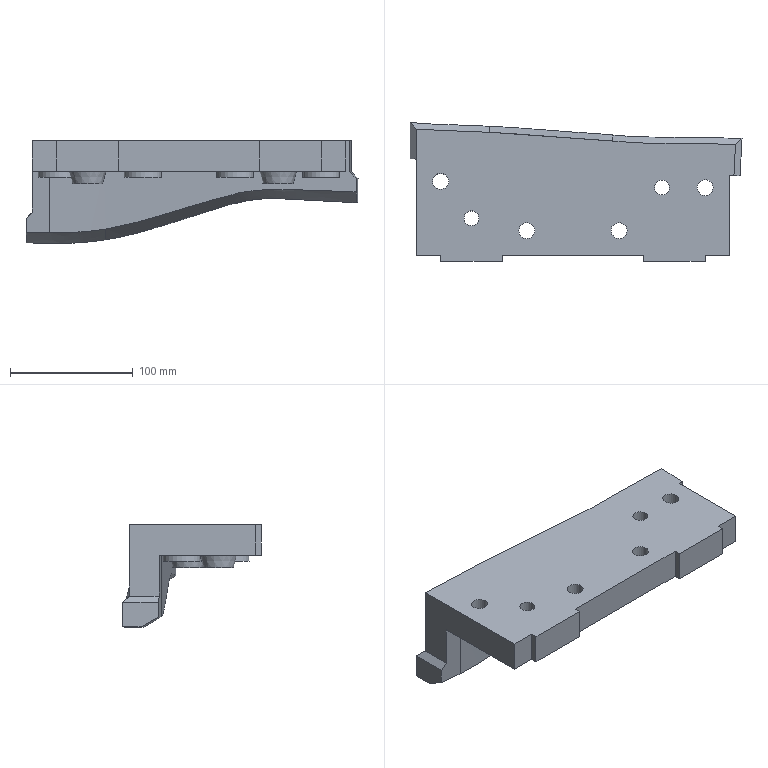Part | NX | features solid 2 | 1 solid | 60 faces | box 270 x 112.969 x 83.658 mm | volume 891046 mm3 | plane 29 | spline 17 | cylinder 12 | cone 2 | commonest cylinder face diameters 13 x6 30 x4 12 x2